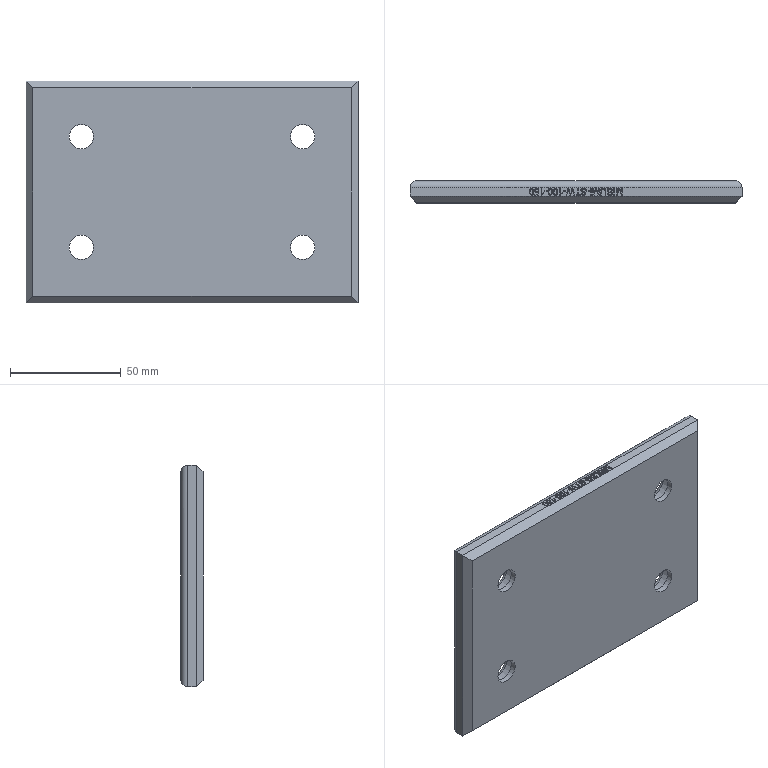Part | NX | features FD 2 | 1 solid | 171 faces | box 150 x 10 x 100 mm | volume 138461 mm3 | plane 116 | spline 39 | cylinder 12 | torus 4 | commonest cylinder face diameters 6 x4 11 x4 17.5 x4